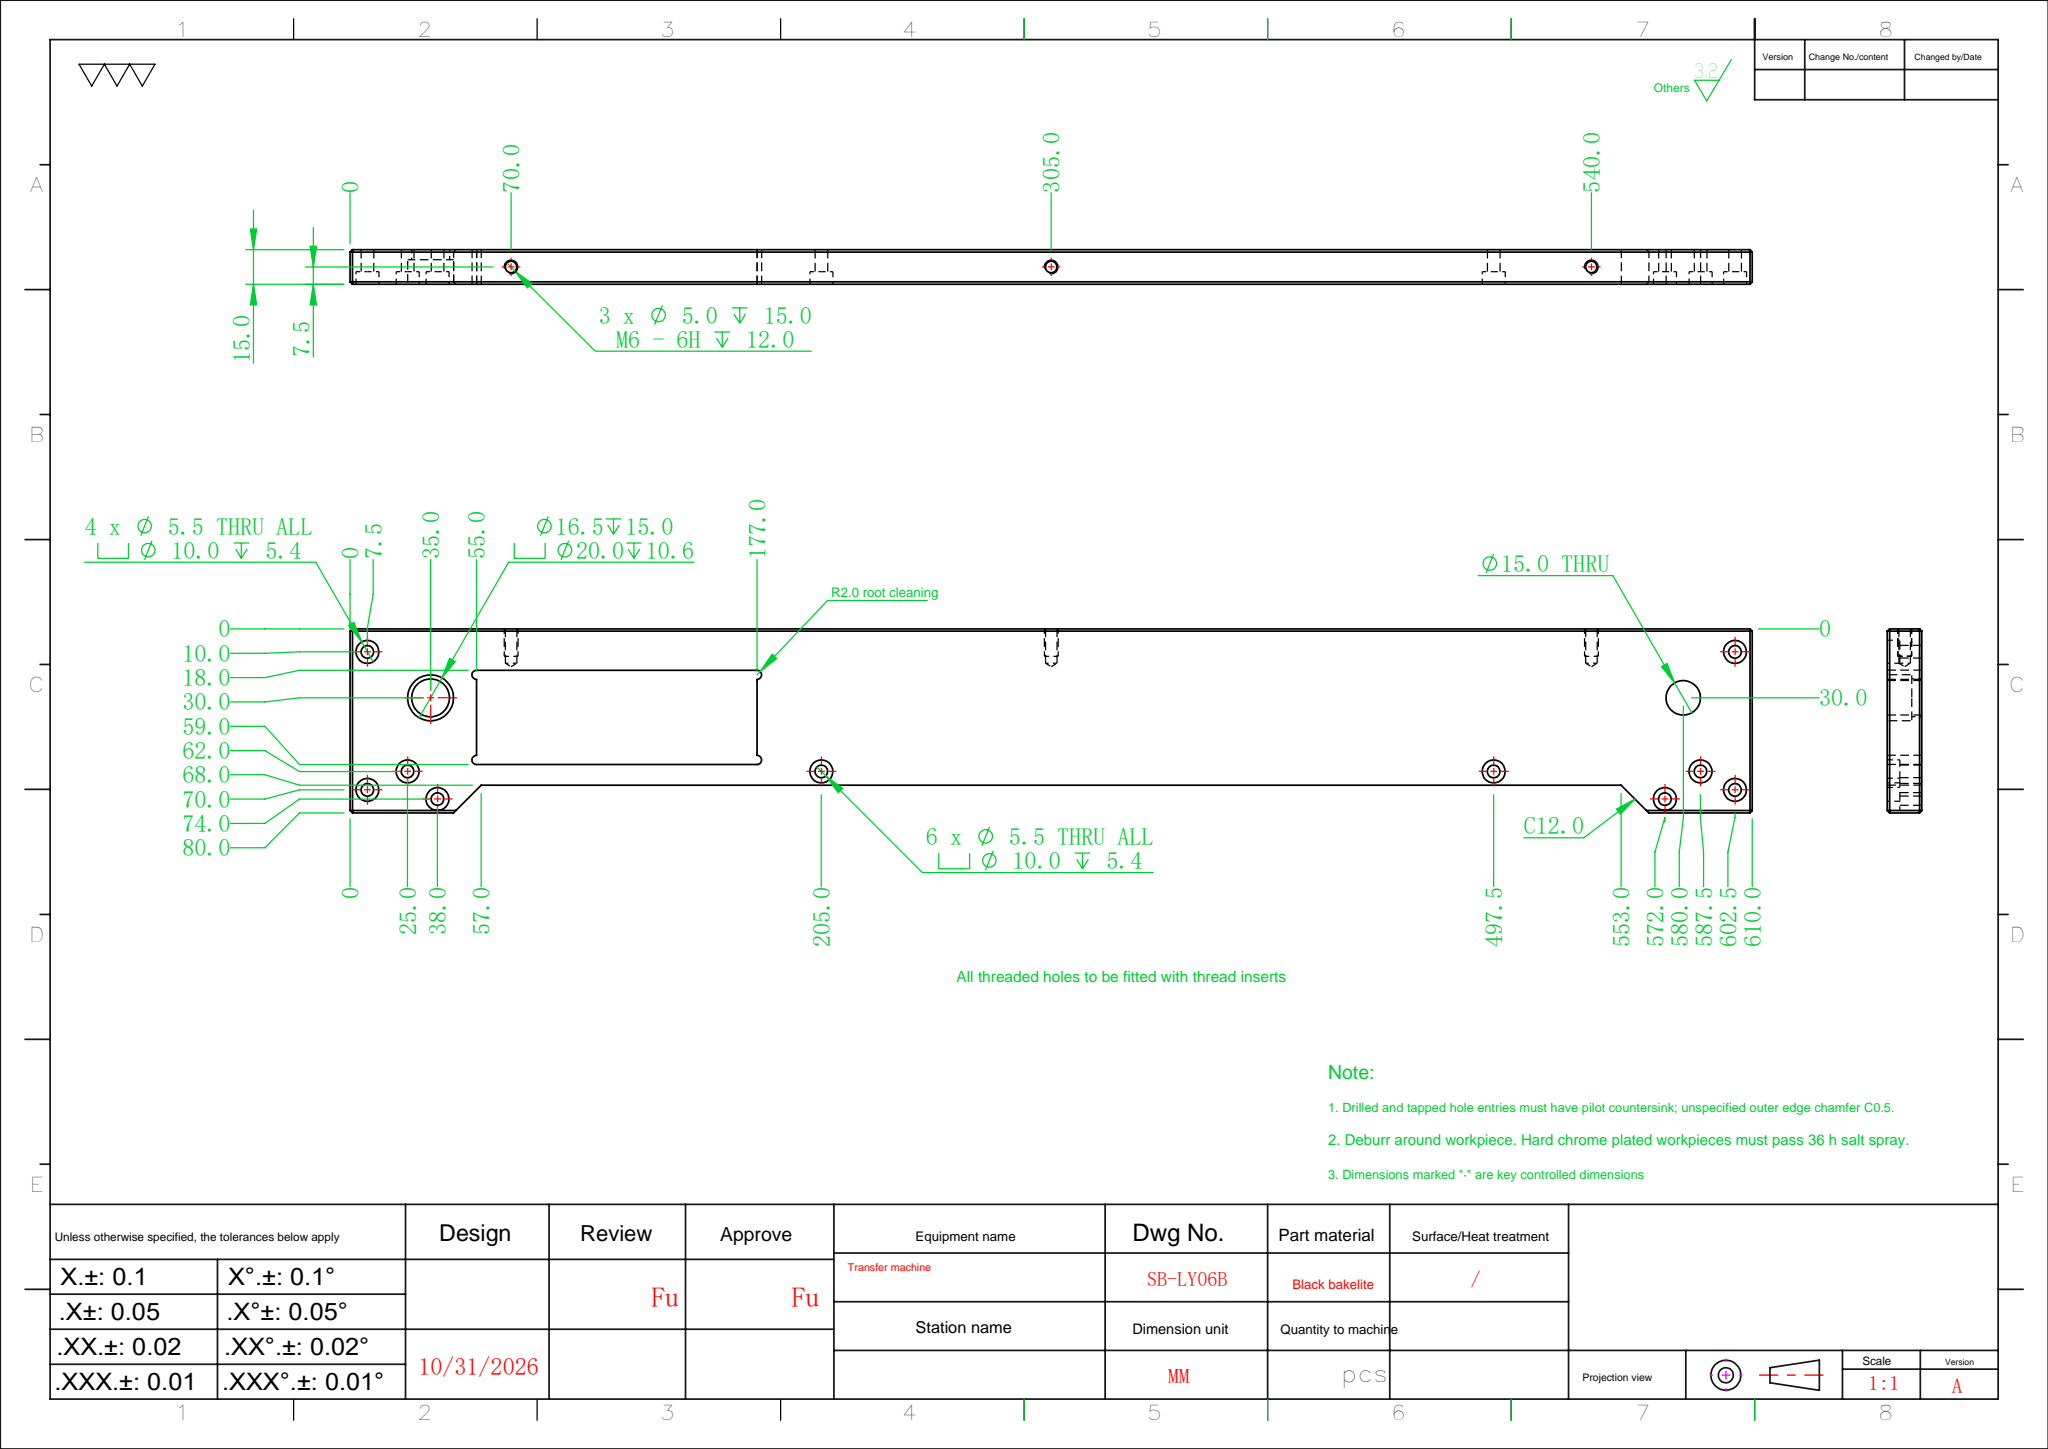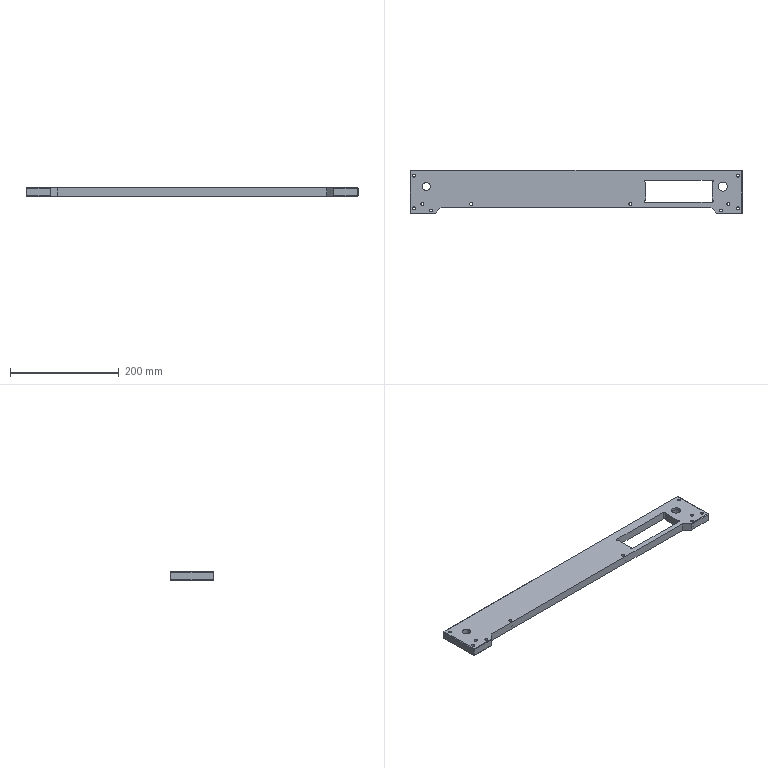Part | SolidWorks | features Cut 5, HoleWzd 3, Chamfer 2, Extrusion 1, ICE 1 | 1 solid | 111 faces | box 610 x 80 x 15 mm | volume 549911 mm3 | cylinder 58 | plane 47 | cone 6 | commonest cylinder face diameters 5.5 x20 10 x20 4 x6 5 x6 15 x2 16.5 x2